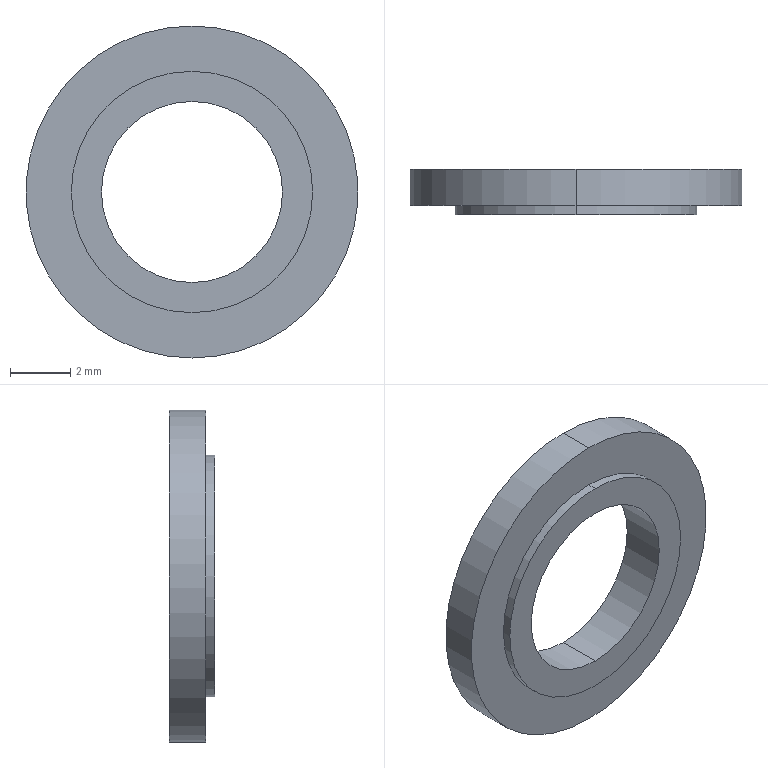Part | NX | features BREP 1 | 1 solid | 9 faces | box 11 x 1.5 x 11 mm | volume 86.708 mm3 | cylinder 6 | plane 3 | commonest cylinder face diameters 6 x2 8 x2 11 x2
STEP:
#1=CARTESIAN_POINT('',(0.,1.5,-3.));
#2=VERTEX_POINT('',#1);
#3=CARTESIAN_POINT('',(0.,1.5,3.));
#4=VERTEX_POINT('',#3);
#5=CARTESIAN_POINT('',(0.,1.5,0.));
#6=DIRECTION('',(0.,-1.,0.));
#7=DIRECTION('',(0.,0.,-1.));
#8=AXIS2_PLACEMENT_3D('',#5,#6,#7);
#9=CIRCLE('',#8,3.);
#10=EDGE_CURVE('',#2,#4,#9,.T.);
#11=ORIENTED_EDGE('',*,*,#10,.T.);
#12=CARTESIAN_POINT('',(0.,1.5,0.));
#13=DIRECTION('',(0.,-1.,0.));
#14=DIRECTION('',(0.,0.,-1.));
#15=AXIS2_PLACEMENT_3D('',#12,#13,#14);
#16=CIRCLE('',#15,3.);
#17=EDGE_CURVE('',#4,#2,#16,.T.);
#18=ORIENTED_EDGE('',*,*,#17,.T.);
#19=EDGE_LOOP('',(#11,#18));
#20=FACE_BOUND('',#19,.T.);
#21=CARTESIAN_POINT('',(0.,1.5,-5.5));
#22=VERTEX_POINT('',#21);
#23=CARTESIAN_POINT('',(0.,1.5,5.5));
#24=VERTEX_POINT('',#23);
#25=CARTESIAN_POINT('',(0.,1.5,0.));
#26=DIRECTION('',(0.,-1.,0.));
#27=DIRECTION('',(0.,0.,-1.));
#28=AXIS2_PLACEMENT_3D('',#25,#26,#27);
#29=CIRCLE('',#28,5.5);
#30=EDGE_CURVE('',#22,#24,#29,.T.);
#31=ORIENTED_EDGE('',*,*,#30,.F.);
#32=CARTESIAN_POINT('',(0.,1.5,0.));
#33=DIRECTION('',(0.,-1.,0.));
#34=DIRECTION('',(0.,0.,-1.));
#35=AXIS2_PLACEMENT_3D('',#32,#33,#34);
#36=CIRCLE('',#35,5.5);
#37=EDGE_CURVE('',#24,#22,#36,.T.);
#38=ORIENTED_EDGE('',*,*,#37,.F.);
#39=EDGE_LOOP('',(#31,#38));
#40=FACE_BOUND('',#39,.T.);
#41=CARTESIAN_POINT('',(-5.5,1.5,0.));
#42=DIRECTION('',(0.,-1.,0.));
#43=DIRECTION('',(0.,0.,-1.));
#44=AXIS2_PLACEMENT_3D('',#41,#42,#43);
#45=PLANE('',#44);
#46=ADVANCED_FACE('',(#20,#40),#45,.F.);
#47=CARTESIAN_POINT('',(0.,0.3,5.5));
#48=VERTEX_POINT('',#47);
#49=CARTESIAN_POINT('',(0.,0.,5.5));
#50=DIRECTION('',(0.,-1.,0.));
#51=VECTOR('',#50,1000.);
#52=LINE('',#49,#51);
#53=EDGE_CURVE('',#24,#48,#52,.T.);
#54=ORIENTED_EDGE('',*,*,#53,.F.);
#55=ORIENTED_EDGE('',*,*,#37,.T.);
#56=CARTESIAN_POINT('',(0.,0.3,-5.5));
#57=VERTEX_POINT('',#56);
#58=CARTESIAN_POINT('',(0.,0.,-5.5));
#59=DIRECTION('',(0.,-1.,0.));
#60=VECTOR('',#59,1000.);
#61=LINE('',#58,#60);
#62=EDGE_CURVE('',#22,#57,#61,.T.);
#63=ORIENTED_EDGE('',*,*,#62,.T.);
#64=CARTESIAN_POINT('',(0.,0.3,0.));
#65=DIRECTION('',(0.,-1.,0.));
#66=DIRECTION('',(0.,0.,-1.));
#67=AXIS2_PLACEMENT_3D('',#64,#65,#66);
#68=CIRCLE('',#67,5.5);
#69=EDGE_CURVE('',#48,#57,#68,.T.);
#70=ORIENTED_EDGE('',*,*,#69,.F.);
#71=EDGE_LOOP('',(#54,#55,#63,#70));
#72=FACE_BOUND('',#71,.T.);
#73=CARTESIAN_POINT('',(0.,0.,0.));
#74=DIRECTION('',(0.,-1.,0.));
#75=DIRECTION('',(0.,0.,-1.));
#76=AXIS2_PLACEMENT_3D('',#73,#74,#75);
#77=CYLINDRICAL_SURFACE('',#76,5.5);
#78=ADVANCED_FACE('',(#72),#77,.T.);
#79=CARTESIAN_POINT('',(0.,0.3,0.));
#80=DIRECTION('',(0.,-1.,0.));
#81=DIRECTION('',(0.,0.,-1.));
#82=AXIS2_PLACEMENT_3D('',#79,#80,#81);
#83=CIRCLE('',#82,5.5);
#84=EDGE_CURVE('',#57,#48,#83,.T.);
#85=ORIENTED_EDGE('',*,*,#84,.T.);
#86=ORIENTED_EDGE('',*,*,#69,.T.);
#87=EDGE_LOOP('',(#85,#86));
#88=FACE_BOUND('',#87,.T.);
#89=CARTESIAN_POINT('',(0.,0.3,-4.));
#90=VERTEX_POINT('',#89);
#91=CARTESIAN_POINT('',(0.,0.3,4.));
#92=VERTEX_POINT('',#91);
#93=CARTESIAN_POINT('',(0.,0.3,0.));
#94=DIRECTION('',(0.,-1.,0.));
#95=DIRECTION('',(0.,0.,-1.));
#96=AXIS2_PLACEMENT_3D('',#93,#94,#95);
#97=CIRCLE('',#96,4.);
#98=EDGE_CURVE('',#90,#92,#97,.T.);
#99=ORIENTED_EDGE('',*,*,#98,.F.);
#100=CARTESIAN_POINT('',(0.,0.3,0.));
#101=DIRECTION('',(0.,-1.,0.));
#102=DIRECTION('',(0.,0.,-1.));
#103=AXIS2_PLACEMENT_3D('',#100,#101,#102);
#104=CIRCLE('',#103,4.);
#105=EDGE_CURVE('',#92,#90,#104,.T.);
#106=ORIENTED_EDGE('',*,*,#105,.F.);
#107=EDGE_LOOP('',(#99,#106));
#108=FACE_BOUND('',#107,.T.);
#109=CARTESIAN_POINT('',(-4.,0.3,0.));
#110=DIRECTION('',(0.,1.,0.));
#111=DIRECTION('',(0.,0.,1.));
#112=AXIS2_PLACEMENT_3D('',#109,#110,#111);
#113=PLANE('',#112);
#114=ADVANCED_FACE('',(#88,#108),#113,.F.);
#115=CARTESIAN_POINT('',(0.,0.,4.));
#116=VERTEX_POINT('',#115);
#117=CARTESIAN_POINT('',(0.,0.,4.));
#118=DIRECTION('',(0.,-1.,0.));
#119=VECTOR('',#118,1000.);
#120=LINE('',#117,#119);
#121=EDGE_CURVE('',#92,#116,#120,.T.);
#122=ORIENTED_EDGE('',*,*,#121,.F.);
#123=ORIENTED_EDGE('',*,*,#105,.T.);
#124=CARTESIAN_POINT('',(0.,0.,-4.));
#125=VERTEX_POINT('',#124);
#126=CARTESIAN_POINT('',(0.,0.,-4.));
#127=DIRECTION('',(0.,-1.,0.));
#128=VECTOR('',#127,1000.);
#129=LINE('',#126,#128);
#130=EDGE_CURVE('',#90,#125,#129,.T.);
#131=ORIENTED_EDGE('',*,*,#130,.T.);
#132=CARTESIAN_POINT('',(0.,0.,0.));
#133=DIRECTION('',(0.,-1.,0.));
#134=DIRECTION('',(0.,0.,-1.));
#135=AXIS2_PLACEMENT_3D('',#132,#133,#134);
#136=CIRCLE('',#135,4.);
#137=EDGE_CURVE('',#116,#125,#136,.T.);
#138=ORIENTED_EDGE('',*,*,#137,.F.);
#139=EDGE_LOOP('',(#122,#123,#131,#138));
#140=FACE_BOUND('',#139,.T.);
#141=CARTESIAN_POINT('',(0.,0.,0.));
#142=DIRECTION('',(0.,-1.,0.));
#143=DIRECTION('',(0.,0.,-1.));
#144=AXIS2_PLACEMENT_3D('',#141,#142,#143);
#145=CYLINDRICAL_SURFACE('',#144,4.);
#146=ADVANCED_FACE('',(#140),#145,.T.);
#147=CARTESIAN_POINT('',(0.,0.,0.));
#148=DIRECTION('',(0.,-1.,0.));
#149=DIRECTION('',(0.,0.,-1.));
#150=AXIS2_PLACEMENT_3D('',#147,#148,#149);
#151=CIRCLE('',#150,4.);
#152=EDGE_CURVE('',#125,#116,#151,.T.);
#153=ORIENTED_EDGE('',*,*,#152,.T.);
#154=ORIENTED_EDGE('',*,*,#137,.T.);
#155=EDGE_LOOP('',(#153,#154));
#156=FACE_BOUND('',#155,.T.);
#157=CARTESIAN_POINT('',(0.,0.,-3.));
#158=VERTEX_POINT('',#157);
#159=CARTESIAN_POINT('',(0.,0.,3.));
#160=VERTEX_POINT('',#159);
#161=CARTESIAN_POINT('',(0.,0.,0.));
#162=DIRECTION('',(0.,-1.,0.));
#163=DIRECTION('',(0.,0.,-1.));
#164=AXIS2_PLACEMENT_3D('',#161,#162,#163);
#165=CIRCLE('',#164,3.);
#166=EDGE_CURVE('',#158,#160,#165,.T.);
#167=ORIENTED_EDGE('',*,*,#166,.F.);
#168=CARTESIAN_POINT('',(0.,0.,0.));
#169=DIRECTION('',(0.,-1.,0.));
#170=DIRECTION('',(0.,0.,-1.));
#171=AXIS2_PLACEMENT_3D('',#168,#169,#170);
#172=CIRCLE('',#171,3.);
#173=EDGE_CURVE('',#160,#158,#172,.T.);
#174=ORIENTED_EDGE('',*,*,#173,.F.);
#175=EDGE_LOOP('',(#167,#174));
#176=FACE_BOUND('',#175,.T.);
#177=CARTESIAN_POINT('',(-3.,0.,0.));
#178=DIRECTION('',(0.,1.,0.));
#179=DIRECTION('',(0.,0.,1.));
#180=AXIS2_PLACEMENT_3D('',#177,#178,#179);
#181=PLANE('',#180);
#182=ADVANCED_FACE('',(#156,#176),#181,.F.);
#183=CARTESIAN_POINT('',(0.,0.,3.));
#184=DIRECTION('',(0.,-1.,0.));
#185=VECTOR('',#184,1000.);
#186=LINE('',#183,#185);
#187=EDGE_CURVE('',#4,#160,#186,.T.);
#188=ORIENTED_EDGE('',*,*,#187,.F.);
#189=ORIENTED_EDGE('',*,*,#10,.F.);
#190=CARTESIAN_POINT('',(0.,0.,-3.));
#191=DIRECTION('',(0.,-1.,0.));
#192=VECTOR('',#191,1000.);
#193=LINE('',#190,#192);
#194=EDGE_CURVE('',#2,#158,#193,.T.);
#195=ORIENTED_EDGE('',*,*,#194,.T.);
#196=ORIENTED_EDGE('',*,*,#166,.T.);
#197=EDGE_LOOP('',(#188,#189,#195,#196));
#198=FACE_BOUND('',#197,.T.);
#199=CARTESIAN_POINT('',(0.,0.,0.));
#200=DIRECTION('',(0.,-1.,0.));
#201=DIRECTION('',(0.,0.,-1.));
#202=AXIS2_PLACEMENT_3D('',#199,#200,#201);
#203=CYLINDRICAL_SURFACE('',#202,3.);
#204=ADVANCED_FACE('',(#198),#203,.F.);
#205=ORIENTED_EDGE('',*,*,#17,.F.);
#206=ORIENTED_EDGE('',*,*,#187,.T.);
#207=ORIENTED_EDGE('',*,*,#173,.T.);
#208=ORIENTED_EDGE('',*,*,#194,.F.);
#209=EDGE_LOOP('',(#205,#206,#207,#208));
#210=FACE_BOUND('',#209,.T.);
#211=CARTESIAN_POINT('',(0.,0.,0.));
#212=DIRECTION('',(0.,-1.,0.));
#213=DIRECTION('',(0.,0.,-1.));
#214=AXIS2_PLACEMENT_3D('',#211,#212,#213);
#215=CYLINDRICAL_SURFACE('',#214,3.);
#216=ADVANCED_FACE('',(#210),#215,.F.);
#217=ORIENTED_EDGE('',*,*,#98,.T.);
#218=ORIENTED_EDGE('',*,*,#121,.T.);
#219=ORIENTED_EDGE('',*,*,#152,.F.);
#220=ORIENTED_EDGE('',*,*,#130,.F.);
#221=EDGE_LOOP('',(#217,#218,#219,#220));
#222=FACE_BOUND('',#221,.T.);
#223=CARTESIAN_POINT('',(0.,0.,0.));
#224=DIRECTION('',(0.,-1.,0.));
#225=DIRECTION('',(0.,0.,-1.));
#226=AXIS2_PLACEMENT_3D('',#223,#224,#225);
#227=CYLINDRICAL_SURFACE('',#226,4.);
#228=ADVANCED_FACE('',(#222),#227,.T.);
#229=ORIENTED_EDGE('',*,*,#30,.T.);
#230=ORIENTED_EDGE('',*,*,#53,.T.);
#231=ORIENTED_EDGE('',*,*,#84,.F.);
#232=ORIENTED_EDGE('',*,*,#62,.F.);
#233=EDGE_LOOP('',(#229,#230,#231,#232));
#234=FACE_BOUND('',#233,.T.);
#235=CARTESIAN_POINT('',(0.,0.,0.));
#236=DIRECTION('',(0.,-1.,0.));
#237=DIRECTION('',(0.,0.,-1.));
#238=AXIS2_PLACEMENT_3D('',#235,#236,#237);
#239=CYLINDRICAL_SURFACE('',#238,5.5);
#240=ADVANCED_FACE('',(#234),#239,.T.);
#241=CLOSED_SHELL('',(#46,#78,#114,#146,#182,#204,#216,#228,#240));
#242=MANIFOLD_SOLID_BREP('',#241);
#243=(LENGTH_UNIT()NAMED_UNIT(*)SI_UNIT(.MILLI.,.METRE.));
#244=UNCERTAINTY_MEASURE_WITH_UNIT(LENGTH_MEASURE(0.00001),#243,'','');
#245=(NAMED_UNIT(*)PLANE_ANGLE_UNIT()SI_UNIT($,.RADIAN.));
#246=(NAMED_UNIT(*)SI_UNIT($,.STERADIAN.)SOLID_ANGLE_UNIT());
#247=(GEOMETRIC_REPRESENTATION_CONTEXT(3)GLOBAL_UNCERTAINTY_ASSIGNED_CONTEXT((#244))GLOBAL_UNIT_ASSIGNED_CONTEXT((#243,#245,#246))REPRESENTATION_CONTEXT('',''));
#248=ADVANCED_BREP_SHAPE_REPRESENTATION('',(#242),#247);